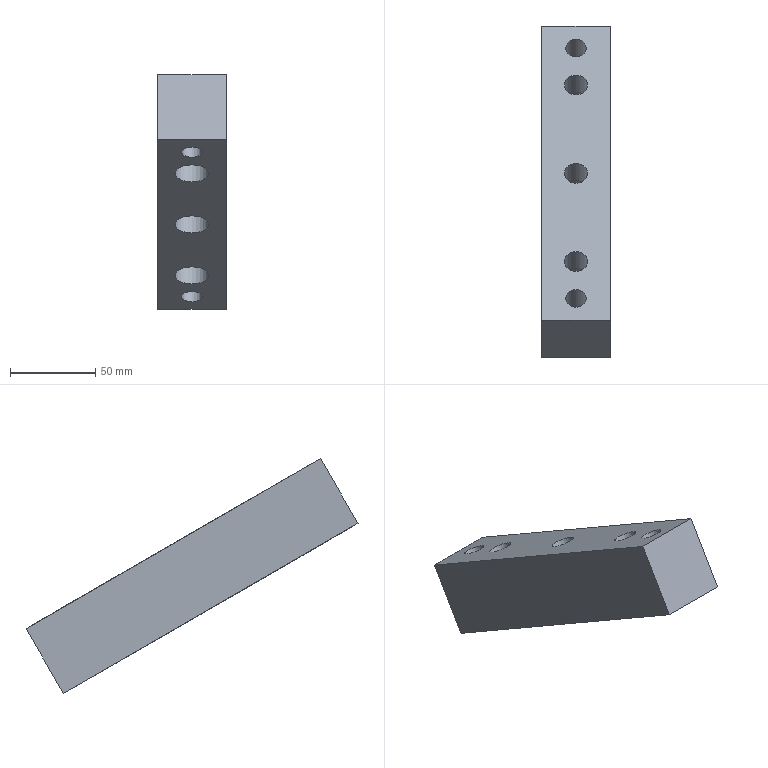Part | NX | features solid 2 | 1 solid | 17 faces | box 40 x 195.205 x 138.105 mm | volume 310840 mm3 | plane 9 | cylinder 8 | commonest cylinder face diameters 13.5 x3 20 x3 12 x2
STEP:
#1=CARTESIAN_POINT('',(20.,838.231,-24.867));
#2=VERTEX_POINT('',#1);
#3=CARTESIAN_POINT('',(20.,816.231,-62.972));
#4=VERTEX_POINT('',#3);
#5=CARTESIAN_POINT('',(20.,838.231,-24.867));
#6=DIRECTION('',(0.,0.5,0.866));
#7=VECTOR('',#6,1000.);
#8=LINE('',#5,#7);
#9=EDGE_CURVE('',#2,#4,#8,.F.);
#10=ORIENTED_EDGE('',*,*,#9,.T.);
#11=CARTESIAN_POINT('',(20.,989.436,-162.972));
#12=VERTEX_POINT('',#11);
#13=CARTESIAN_POINT('',(20.,823.011,-66.887));
#14=DIRECTION('',(0.,-0.866,0.5));
#15=VECTOR('',#14,1000.);
#16=LINE('',#13,#15);
#17=EDGE_CURVE('',#4,#12,#16,.F.);
#18=ORIENTED_EDGE('',*,*,#17,.T.);
#19=CARTESIAN_POINT('',(20.,1011.436,-124.867));
#20=VERTEX_POINT('',#19);
#21=CARTESIAN_POINT('',(20.,1000.436,-143.919));
#22=DIRECTION('',(0.,0.5,0.866));
#23=VECTOR('',#22,1000.);
#24=LINE('',#21,#23);
#25=EDGE_CURVE('',#20,#12,#24,.F.);
#26=ORIENTED_EDGE('',*,*,#25,.F.);
#27=CARTESIAN_POINT('',(20.,845.011,-28.781));
#28=DIRECTION('',(0.,0.866,-0.5));
#29=VECTOR('',#28,1000.);
#30=LINE('',#27,#29);
#31=EDGE_CURVE('',#2,#20,#30,.T.);
#32=ORIENTED_EDGE('',*,*,#31,.F.);
#33=EDGE_LOOP('',(#10,#18,#26,#32));
#34=FACE_BOUND('',#33,.T.);
#35=CARTESIAN_POINT('',(20.,845.011,-28.781));
#36=DIRECTION('',(1.,0.,0.));
#37=DIRECTION('',(0.,0.866,-0.5));
#38=AXIS2_PLACEMENT_3D('',#35,#36,#37);
#39=PLANE('',#38);
#40=ADVANCED_FACE('',(#34),#39,.T.);
#41=ORIENTED_EDGE('',*,*,#25,.T.);
#42=CARTESIAN_POINT('',(-20.,989.436,-162.972));
#43=VERTEX_POINT('',#42);
#44=CARTESIAN_POINT('',(275.,989.436,-162.972));
#45=DIRECTION('',(-1.,0.,0.));
#46=VECTOR('',#45,1000.);
#47=LINE('',#44,#46);
#48=EDGE_CURVE('',#12,#43,#47,.T.);
#49=ORIENTED_EDGE('',*,*,#48,.T.);
#50=CARTESIAN_POINT('',(-20.,1011.436,-124.867));
#51=VERTEX_POINT('',#50);
#52=CARTESIAN_POINT('',(-20.,1011.436,-124.867));
#53=DIRECTION('',(0.,-0.5,-0.866));
#54=VECTOR('',#53,1000.);
#55=LINE('',#52,#54);
#56=EDGE_CURVE('',#51,#43,#55,.T.);
#57=ORIENTED_EDGE('',*,*,#56,.F.);
#58=CARTESIAN_POINT('',(275.,1011.436,-124.867));
#59=DIRECTION('',(-1.,0.,0.));
#60=VECTOR('',#59,1000.);
#61=LINE('',#58,#60);
#62=EDGE_CURVE('',#20,#51,#61,.T.);
#63=ORIENTED_EDGE('',*,*,#62,.F.);
#64=EDGE_LOOP('',(#41,#49,#57,#63));
#65=FACE_BOUND('',#64,.T.);
#66=CARTESIAN_POINT('',(275.,1000.436,-143.919));
#67=DIRECTION('',(0.,-0.866,0.5));
#68=DIRECTION('',(0.,-0.5,-0.866));
#69=AXIS2_PLACEMENT_3D('',#66,#67,#68);
#70=PLANE('',#69);
#71=ADVANCED_FACE('',(#65),#70,.F.);
#72=ORIENTED_EDGE('',*,*,#56,.T.);
#73=CARTESIAN_POINT('',(-20.,816.231,-62.972));
#74=VERTEX_POINT('',#73);
#75=CARTESIAN_POINT('',(-20.,823.011,-66.887));
#76=DIRECTION('',(0.,-0.866,0.5));
#77=VECTOR('',#76,1000.);
#78=LINE('',#75,#77);
#79=EDGE_CURVE('',#74,#43,#78,.F.);
#80=ORIENTED_EDGE('',*,*,#79,.F.);
#81=CARTESIAN_POINT('',(-20.,838.231,-24.867));
#82=VERTEX_POINT('',#81);
#83=CARTESIAN_POINT('',(-20.,838.231,-24.867));
#84=DIRECTION('',(0.,-0.5,-0.866));
#85=VECTOR('',#84,1000.);
#86=LINE('',#83,#85);
#87=EDGE_CURVE('',#82,#74,#86,.T.);
#88=ORIENTED_EDGE('',*,*,#87,.F.);
#89=CARTESIAN_POINT('',(-20.,845.011,-28.781));
#90=DIRECTION('',(0.,0.866,-0.5));
#91=VECTOR('',#90,1000.);
#92=LINE('',#89,#91);
#93=EDGE_CURVE('',#82,#51,#92,.T.);
#94=ORIENTED_EDGE('',*,*,#93,.T.);
#95=EDGE_LOOP('',(#72,#80,#88,#94));
#96=FACE_BOUND('',#95,.T.);
#97=CARTESIAN_POINT('',(-20.,845.011,-28.781));
#98=DIRECTION('',(1.,0.,0.));
#99=DIRECTION('',(0.,0.866,-0.5));
#100=AXIS2_PLACEMENT_3D('',#97,#98,#99);
#101=PLANE('',#100);
#102=ADVANCED_FACE('',(#96),#101,.F.);
#103=CARTESIAN_POINT('',(20.,838.231,-24.867));
#104=DIRECTION('',(-1.,0.,0.));
#105=VECTOR('',#104,1000.);
#106=LINE('',#103,#105);
#107=EDGE_CURVE('',#2,#82,#106,.T.);
#108=ORIENTED_EDGE('',*,*,#107,.T.);
#109=ORIENTED_EDGE('',*,*,#87,.T.);
#110=CARTESIAN_POINT('',(20.,816.231,-62.972));
#111=DIRECTION('',(-1.,0.,0.));
#112=VECTOR('',#111,1000.);
#113=LINE('',#110,#112);
#114=EDGE_CURVE('',#4,#74,#113,.T.);
#115=ORIENTED_EDGE('',*,*,#114,.F.);
#116=ORIENTED_EDGE('',*,*,#9,.F.);
#117=EDGE_LOOP('',(#108,#109,#115,#116));
#118=FACE_BOUND('',#117,.T.);
#119=CARTESIAN_POINT('',(20.,838.231,-24.867));
#120=DIRECTION('',(0.,0.866,-0.5));
#121=DIRECTION('',(-1.,0.,0.));
#122=AXIS2_PLACEMENT_3D('',#119,#120,#121);
#123=PLANE('',#122);
#124=ADVANCED_FACE('',(#118),#123,.F.);
#125=CARTESIAN_POINT('',(0.,894.173,-107.972));
#126=VERTEX_POINT('',#125);
#127=CARTESIAN_POINT('',(0.,902.833,-112.972));
#128=DIRECTION('',(0.,0.5,0.866));
#129=DIRECTION('',(0.,-0.866,0.5));
#130=AXIS2_PLACEMENT_3D('',#127,#128,#129);
#131=CIRCLE('',#130,10.);
#132=EDGE_CURVE('',#126,#126,#131,.T.);
#133=ORIENTED_EDGE('',*,*,#132,.T.);
#134=EDGE_LOOP('',(#133));
#135=FACE_BOUND('',#134,.T.);
#136=CARTESIAN_POINT('',(0.,842.212,-77.972));
#137=VERTEX_POINT('',#136);
#138=CARTESIAN_POINT('',(0.,850.872,-82.972));
#139=DIRECTION('',(0.,0.5,0.866));
#140=DIRECTION('',(0.,-0.866,0.5));
#141=AXIS2_PLACEMENT_3D('',#138,#139,#140);
#142=CIRCLE('',#141,10.);
#143=EDGE_CURVE('',#137,#137,#142,.T.);
#144=ORIENTED_EDGE('',*,*,#143,.T.);
#145=EDGE_LOOP('',(#144));
#146=FACE_BOUND('',#145,.T.);
#147=CARTESIAN_POINT('',(0.,824.025,-67.472));
#148=VERTEX_POINT('',#147);
#149=CARTESIAN_POINT('',(0.,829.221,-70.472));
#150=DIRECTION('',(0.,0.5,0.866));
#151=DIRECTION('',(0.,-0.866,0.5));
#152=AXIS2_PLACEMENT_3D('',#149,#150,#151);
#153=CIRCLE('',#152,6.);
#154=EDGE_CURVE('',#148,#148,#153,.T.);
#155=ORIENTED_EDGE('',*,*,#154,.T.);
#156=EDGE_LOOP('',(#155));
#157=FACE_BOUND('',#156,.T.);
#158=CARTESIAN_POINT('',(0.,946.135,-137.972));
#159=VERTEX_POINT('',#158);
#160=CARTESIAN_POINT('',(0.,954.795,-142.972));
#161=DIRECTION('',(0.,0.5,0.866));
#162=DIRECTION('',(0.,-0.866,0.5));
#163=AXIS2_PLACEMENT_3D('',#160,#161,#162);
#164=CIRCLE('',#163,10.);
#165=EDGE_CURVE('',#159,#159,#164,.T.);
#166=ORIENTED_EDGE('',*,*,#165,.T.);
#167=EDGE_LOOP('',(#166));
#168=FACE_BOUND('',#167,.T.);
#169=CARTESIAN_POINT('',(0.,971.249,-152.472));
#170=VERTEX_POINT('',#169);
#171=CARTESIAN_POINT('',(0.,976.445,-155.472));
#172=DIRECTION('',(0.,0.5,0.866));
#173=DIRECTION('',(0.,-0.866,0.5));
#174=AXIS2_PLACEMENT_3D('',#171,#172,#173);
#175=CIRCLE('',#174,6.);
#176=EDGE_CURVE('',#170,#170,#175,.T.);
#177=ORIENTED_EDGE('',*,*,#176,.T.);
#178=EDGE_LOOP('',(#177));
#179=FACE_BOUND('',#178,.T.);
#180=ORIENTED_EDGE('',*,*,#79,.T.);
#181=ORIENTED_EDGE('',*,*,#48,.F.);
#182=ORIENTED_EDGE('',*,*,#17,.F.);
#183=ORIENTED_EDGE('',*,*,#114,.T.);
#184=EDGE_LOOP('',(#180,#181,#182,#183));
#185=FACE_BOUND('',#184,.T.);
#186=CARTESIAN_POINT('',(20.,823.011,-66.887));
#187=DIRECTION('',(0.,0.5,0.866));
#188=DIRECTION('',(0.,-0.866,0.5));
#189=AXIS2_PLACEMENT_3D('',#186,#187,#188);
#190=PLANE('',#189);
#191=ADVANCED_FACE('',(#135,#146,#157,#168,#179,#185),#190,.F.);
#192=CARTESIAN_POINT('',(0.,918.988,-71.492));
#193=VERTEX_POINT('',#192);
#194=CARTESIAN_POINT('',(0.,924.833,-74.867));
#195=DIRECTION('',(0.,0.5,0.866));
#196=DIRECTION('',(0.,-0.866,0.5));
#197=AXIS2_PLACEMENT_3D('',#194,#195,#196);
#198=CIRCLE('',#197,6.75);
#199=EDGE_CURVE('',#193,#193,#198,.T.);
#200=ORIENTED_EDGE('',*,*,#199,.F.);
#201=EDGE_LOOP('',(#200));
#202=FACE_BOUND('',#201,.T.);
#203=CARTESIAN_POINT('',(0.,867.026,-41.492));
#204=VERTEX_POINT('',#203);
#205=CARTESIAN_POINT('',(0.,872.872,-44.867));
#206=DIRECTION('',(0.,0.5,0.866));
#207=DIRECTION('',(0.,-0.866,0.5));
#208=AXIS2_PLACEMENT_3D('',#205,#206,#207);
#209=CIRCLE('',#208,6.75);
#210=EDGE_CURVE('',#204,#204,#209,.T.);
#211=ORIENTED_EDGE('',*,*,#210,.F.);
#212=EDGE_LOOP('',(#211));
#213=FACE_BOUND('',#212,.T.);
#214=CARTESIAN_POINT('',(0.,846.025,-29.367));
#215=VERTEX_POINT('',#214);
#216=CARTESIAN_POINT('',(0.,851.221,-32.367));
#217=DIRECTION('',(0.,0.5,0.866));
#218=DIRECTION('',(0.,-0.866,0.5));
#219=AXIS2_PLACEMENT_3D('',#216,#217,#218);
#220=CIRCLE('',#219,6.);
#221=EDGE_CURVE('',#215,#215,#220,.T.);
#222=ORIENTED_EDGE('',*,*,#221,.F.);
#223=EDGE_LOOP('',(#222));
#224=FACE_BOUND('',#223,.T.);
#225=CARTESIAN_POINT('',(0.,970.949,-101.492));
#226=VERTEX_POINT('',#225);
#227=CARTESIAN_POINT('',(0.,976.795,-104.867));
#228=DIRECTION('',(0.,0.5,0.866));
#229=DIRECTION('',(0.,-0.866,0.5));
#230=AXIS2_PLACEMENT_3D('',#227,#228,#229);
#231=CIRCLE('',#230,6.75);
#232=EDGE_CURVE('',#226,#226,#231,.T.);
#233=ORIENTED_EDGE('',*,*,#232,.F.);
#234=EDGE_LOOP('',(#233));
#235=FACE_BOUND('',#234,.T.);
#236=CARTESIAN_POINT('',(0.,993.249,-114.367));
#237=VERTEX_POINT('',#236);
#238=CARTESIAN_POINT('',(0.,998.445,-117.367));
#239=DIRECTION('',(0.,0.5,0.866));
#240=DIRECTION('',(0.,-0.866,0.5));
#241=AXIS2_PLACEMENT_3D('',#238,#239,#240);
#242=CIRCLE('',#241,6.);
#243=EDGE_CURVE('',#237,#237,#242,.T.);
#244=ORIENTED_EDGE('',*,*,#243,.F.);
#245=EDGE_LOOP('',(#244));
#246=FACE_BOUND('',#245,.T.);
#247=ORIENTED_EDGE('',*,*,#93,.F.);
#248=ORIENTED_EDGE('',*,*,#107,.F.);
#249=ORIENTED_EDGE('',*,*,#31,.T.);
#250=ORIENTED_EDGE('',*,*,#62,.T.);
#251=EDGE_LOOP('',(#247,#248,#249,#250));
#252=FACE_BOUND('',#251,.T.);
#253=CARTESIAN_POINT('',(20.,845.011,-28.781));
#254=DIRECTION('',(0.,0.5,0.866));
#255=DIRECTION('',(0.,-0.866,0.5));
#256=AXIS2_PLACEMENT_3D('',#253,#254,#255);
#257=PLANE('',#256);
#258=ADVANCED_FACE('',(#202,#213,#224,#235,#246,#252),#257,.T.);
#259=ORIENTED_EDGE('',*,*,#243,.T.);
#260=EDGE_LOOP('',(#259));
#261=FACE_BOUND('',#260,.T.);
#262=ORIENTED_EDGE('',*,*,#176,.F.);
#263=EDGE_LOOP('',(#262));
#264=FACE_BOUND('',#263,.T.);
#265=CARTESIAN_POINT('',(0.,976.445,-155.472));
#266=DIRECTION('',(0.,0.5,0.866));
#267=DIRECTION('',(0.,-0.866,0.5));
#268=AXIS2_PLACEMENT_3D('',#265,#266,#267);
#269=CYLINDRICAL_SURFACE('',#268,6.);
#270=ADVANCED_FACE('',(#261,#264),#269,.F.);
#271=ORIENTED_EDGE('',*,*,#232,.T.);
#272=EDGE_LOOP('',(#271));
#273=FACE_BOUND('',#272,.T.);
#274=CARTESIAN_POINT('',(0.,960.949,-118.812));
#275=VERTEX_POINT('',#274);
#276=CARTESIAN_POINT('',(0.,966.795,-122.187));
#277=DIRECTION('',(0.,0.5,0.866));
#278=DIRECTION('',(0.,-0.866,0.5));
#279=AXIS2_PLACEMENT_3D('',#276,#277,#278);
#280=CIRCLE('',#279,6.75);
#281=EDGE_CURVE('',#275,#275,#280,.T.);
#282=ORIENTED_EDGE('',*,*,#281,.F.);
#283=EDGE_LOOP('',(#282));
#284=FACE_BOUND('',#283,.T.);
#285=CARTESIAN_POINT('',(0.,1004.795,-56.369));
#286=DIRECTION('',(0.,0.5,0.866));
#287=DIRECTION('',(0.,-0.866,0.5));
#288=AXIS2_PLACEMENT_3D('',#285,#286,#287);
#289=CYLINDRICAL_SURFACE('',#288,6.75);
#290=ADVANCED_FACE('',(#273,#284),#289,.F.);
#291=ORIENTED_EDGE('',*,*,#281,.T.);
#292=EDGE_LOOP('',(#291));
#293=FACE_BOUND('',#292,.T.);
#294=CARTESIAN_POINT('',(0.,958.135,-117.187));
#295=VERTEX_POINT('',#294);
#296=CARTESIAN_POINT('',(0.,966.795,-122.187));
#297=DIRECTION('',(0.,0.5,0.866));
#298=DIRECTION('',(0.,-0.866,0.5));
#299=AXIS2_PLACEMENT_3D('',#296,#297,#298);
#300=CIRCLE('',#299,10.);
#301=EDGE_CURVE('',#295,#295,#300,.T.);
#302=ORIENTED_EDGE('',*,*,#301,.F.);
#303=EDGE_LOOP('',(#302));
#304=FACE_BOUND('',#303,.T.);
#305=CARTESIAN_POINT('',(0.,966.795,-122.187));
#306=DIRECTION('',(0.,0.5,0.866));
#307=DIRECTION('',(0.,-0.866,0.5));
#308=AXIS2_PLACEMENT_3D('',#305,#306,#307);
#309=PLANE('',#308);
#310=ADVANCED_FACE('',(#293,#304),#309,.F.);
#311=ORIENTED_EDGE('',*,*,#301,.T.);
#312=EDGE_LOOP('',(#311));
#313=FACE_BOUND('',#312,.T.);
#314=ORIENTED_EDGE('',*,*,#165,.F.);
#315=EDGE_LOOP('',(#314));
#316=FACE_BOUND('',#315,.T.);
#317=CARTESIAN_POINT('',(0.,954.795,-142.972));
#318=DIRECTION('',(0.,0.5,0.866));
#319=DIRECTION('',(0.,-0.866,0.5));
#320=AXIS2_PLACEMENT_3D('',#317,#318,#319);
#321=CYLINDRICAL_SURFACE('',#320,10.);
#322=ADVANCED_FACE('',(#313,#316),#321,.F.);
#323=ORIENTED_EDGE('',*,*,#221,.T.);
#324=EDGE_LOOP('',(#323));
#325=FACE_BOUND('',#324,.T.);
#326=ORIENTED_EDGE('',*,*,#154,.F.);
#327=EDGE_LOOP('',(#326));
#328=FACE_BOUND('',#327,.T.);
#329=CARTESIAN_POINT('',(0.,829.221,-70.472));
#330=DIRECTION('',(0.,0.5,0.866));
#331=DIRECTION('',(0.,-0.866,0.5));
#332=AXIS2_PLACEMENT_3D('',#329,#330,#331);
#333=CYLINDRICAL_SURFACE('',#332,6.);
#334=ADVANCED_FACE('',(#325,#328),#333,.F.);
#335=ORIENTED_EDGE('',*,*,#210,.T.);
#336=EDGE_LOOP('',(#335));
#337=FACE_BOUND('',#336,.T.);
#338=CARTESIAN_POINT('',(0.,857.026,-58.812));
#339=VERTEX_POINT('',#338);
#340=CARTESIAN_POINT('',(0.,862.872,-62.187));
#341=DIRECTION('',(0.,0.5,0.866));
#342=DIRECTION('',(0.,-0.866,0.5));
#343=AXIS2_PLACEMENT_3D('',#340,#341,#342);
#344=CIRCLE('',#343,6.75);
#345=EDGE_CURVE('',#339,#339,#344,.T.);
#346=ORIENTED_EDGE('',*,*,#345,.F.);
#347=EDGE_LOOP('',(#346));
#348=FACE_BOUND('',#347,.T.);
#349=CARTESIAN_POINT('',(0.,900.872,3.631));
#350=DIRECTION('',(0.,0.5,0.866));
#351=DIRECTION('',(0.,-0.866,0.5));
#352=AXIS2_PLACEMENT_3D('',#349,#350,#351);
#353=CYLINDRICAL_SURFACE('',#352,6.75);
#354=ADVANCED_FACE('',(#337,#348),#353,.F.);
#355=ORIENTED_EDGE('',*,*,#345,.T.);
#356=EDGE_LOOP('',(#355));
#357=FACE_BOUND('',#356,.T.);
#358=CARTESIAN_POINT('',(0.,854.212,-57.187));
#359=VERTEX_POINT('',#358);
#360=CARTESIAN_POINT('',(0.,862.872,-62.187));
#361=DIRECTION('',(0.,0.5,0.866));
#362=DIRECTION('',(0.,-0.866,0.5));
#363=AXIS2_PLACEMENT_3D('',#360,#361,#362);
#364=CIRCLE('',#363,10.);
#365=EDGE_CURVE('',#359,#359,#364,.T.);
#366=ORIENTED_EDGE('',*,*,#365,.F.);
#367=EDGE_LOOP('',(#366));
#368=FACE_BOUND('',#367,.T.);
#369=CARTESIAN_POINT('',(0.,862.872,-62.187));
#370=DIRECTION('',(0.,0.5,0.866));
#371=DIRECTION('',(0.,-0.866,0.5));
#372=AXIS2_PLACEMENT_3D('',#369,#370,#371);
#373=PLANE('',#372);
#374=ADVANCED_FACE('',(#357,#368),#373,.F.);
#375=ORIENTED_EDGE('',*,*,#365,.T.);
#376=EDGE_LOOP('',(#375));
#377=FACE_BOUND('',#376,.T.);
#378=ORIENTED_EDGE('',*,*,#143,.F.);
#379=EDGE_LOOP('',(#378));
#380=FACE_BOUND('',#379,.T.);
#381=CARTESIAN_POINT('',(0.,850.872,-82.972));
#382=DIRECTION('',(0.,0.5,0.866));
#383=DIRECTION('',(0.,-0.866,0.5));
#384=AXIS2_PLACEMENT_3D('',#381,#382,#383);
#385=CYLINDRICAL_SURFACE('',#384,10.);
#386=ADVANCED_FACE('',(#377,#380),#385,.F.);
#387=ORIENTED_EDGE('',*,*,#199,.T.);
#388=EDGE_LOOP('',(#387));
#389=FACE_BOUND('',#388,.T.);
#390=CARTESIAN_POINT('',(0.,908.988,-88.812));
#391=VERTEX_POINT('',#390);
#392=CARTESIAN_POINT('',(0.,914.833,-92.187));
#393=DIRECTION('',(0.,0.5,0.866));
#394=DIRECTION('',(0.,-0.866,0.5));
#395=AXIS2_PLACEMENT_3D('',#392,#393,#394);
#396=CIRCLE('',#395,6.75);
#397=EDGE_CURVE('',#391,#391,#396,.T.);
#398=ORIENTED_EDGE('',*,*,#397,.F.);
#399=EDGE_LOOP('',(#398));
#400=FACE_BOUND('',#399,.T.);
#401=CARTESIAN_POINT('',(0.,952.833,-26.369));
#402=DIRECTION('',(0.,0.5,0.866));
#403=DIRECTION('',(0.,-0.866,0.5));
#404=AXIS2_PLACEMENT_3D('',#401,#402,#403);
#405=CYLINDRICAL_SURFACE('',#404,6.75);
#406=ADVANCED_FACE('',(#389,#400),#405,.F.);
#407=ORIENTED_EDGE('',*,*,#397,.T.);
#408=EDGE_LOOP('',(#407));
#409=FACE_BOUND('',#408,.T.);
#410=CARTESIAN_POINT('',(0.,906.173,-87.187));
#411=VERTEX_POINT('',#410);
#412=CARTESIAN_POINT('',(0.,914.833,-92.187));
#413=DIRECTION('',(0.,0.5,0.866));
#414=DIRECTION('',(0.,-0.866,0.5));
#415=AXIS2_PLACEMENT_3D('',#412,#413,#414);
#416=CIRCLE('',#415,10.);
#417=EDGE_CURVE('',#411,#411,#416,.T.);
#418=ORIENTED_EDGE('',*,*,#417,.F.);
#419=EDGE_LOOP('',(#418));
#420=FACE_BOUND('',#419,.T.);
#421=CARTESIAN_POINT('',(0.,914.833,-92.187));
#422=DIRECTION('',(0.,0.5,0.866));
#423=DIRECTION('',(0.,-0.866,0.5));
#424=AXIS2_PLACEMENT_3D('',#421,#422,#423);
#425=PLANE('',#424);
#426=ADVANCED_FACE('',(#409,#420),#425,.F.);
#427=ORIENTED_EDGE('',*,*,#417,.T.);
#428=EDGE_LOOP('',(#427));
#429=FACE_BOUND('',#428,.T.);
#430=ORIENTED_EDGE('',*,*,#132,.F.);
#431=EDGE_LOOP('',(#430));
#432=FACE_BOUND('',#431,.T.);
#433=CARTESIAN_POINT('',(0.,902.833,-112.972));
#434=DIRECTION('',(0.,0.5,0.866));
#435=DIRECTION('',(0.,-0.866,0.5));
#436=AXIS2_PLACEMENT_3D('',#433,#434,#435);
#437=CYLINDRICAL_SURFACE('',#436,10.);
#438=ADVANCED_FACE('',(#429,#432),#437,.F.);
#439=CLOSED_SHELL('',(#40,#71,#102,#124,#191,#258,#270,#290,#310,#322,#334,#354,#374,#386,#406,#426,#438));
#440=MANIFOLD_SOLID_BREP('',#439);
#441=(LENGTH_UNIT()NAMED_UNIT(*)SI_UNIT(.MILLI.,.METRE.));
#442=UNCERTAINTY_MEASURE_WITH_UNIT(LENGTH_MEASURE(0.00001),#441,'','');
#443=(NAMED_UNIT(*)PLANE_ANGLE_UNIT()SI_UNIT($,.RADIAN.));
#444=(NAMED_UNIT(*)SI_UNIT($,.STERADIAN.)SOLID_ANGLE_UNIT());
#445=(GEOMETRIC_REPRESENTATION_CONTEXT(3)GLOBAL_UNCERTAINTY_ASSIGNED_CONTEXT((#442))GLOBAL_UNIT_ASSIGNED_CONTEXT((#441,#443,#444))REPRESENTATION_CONTEXT('',''));
#446=ADVANCED_BREP_SHAPE_REPRESENTATION('',(#440),#445);